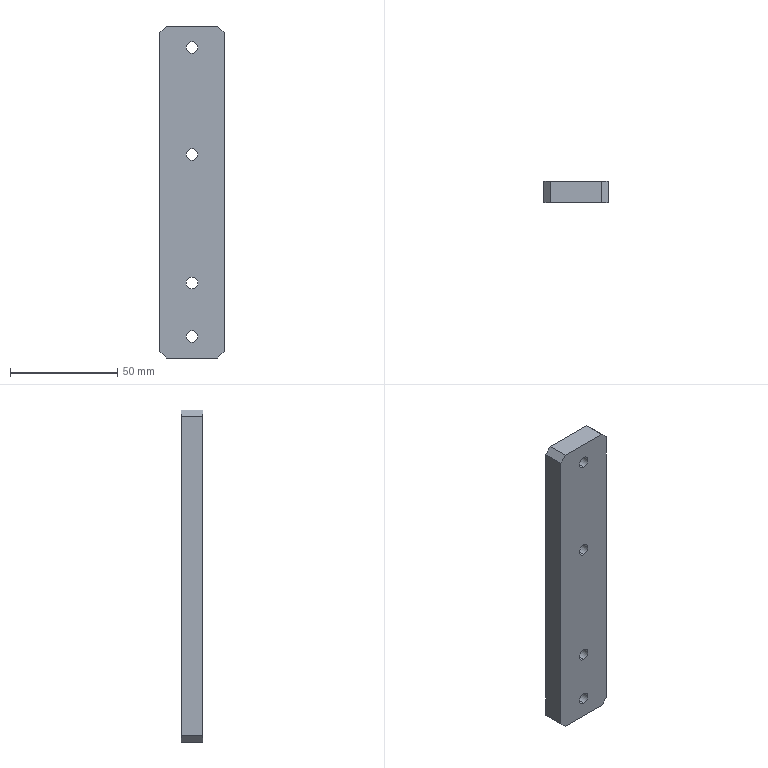Part | STEP file | PN_0023 Connecting block | 1 solid | 30 faces | box 30 x 10 x 155 mm | volume 44164 mm3 | cylinder 16 | plane 14 | commonest cylinder face diameters 5.5 x8 10 x8